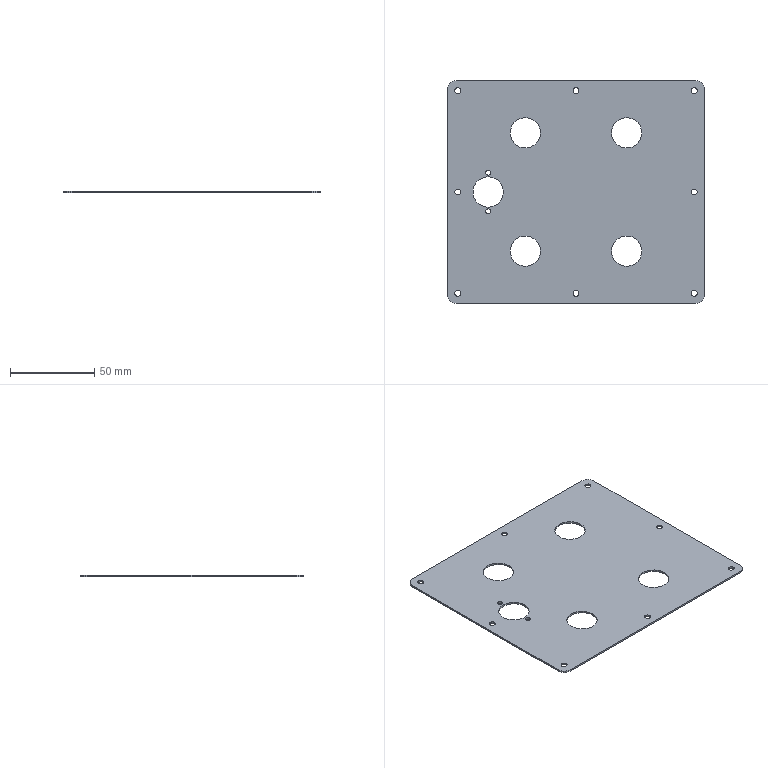Part | STEP file | RJWD-DY-0113--0001 | 1 solid | 40 faces | box 152 x 132 x 1 mm | volume 18679 mm3 | cylinder 34 | plane 6 | commonest cylinder face diameters 3.5 x16 18 x10 3 x4 10 x4